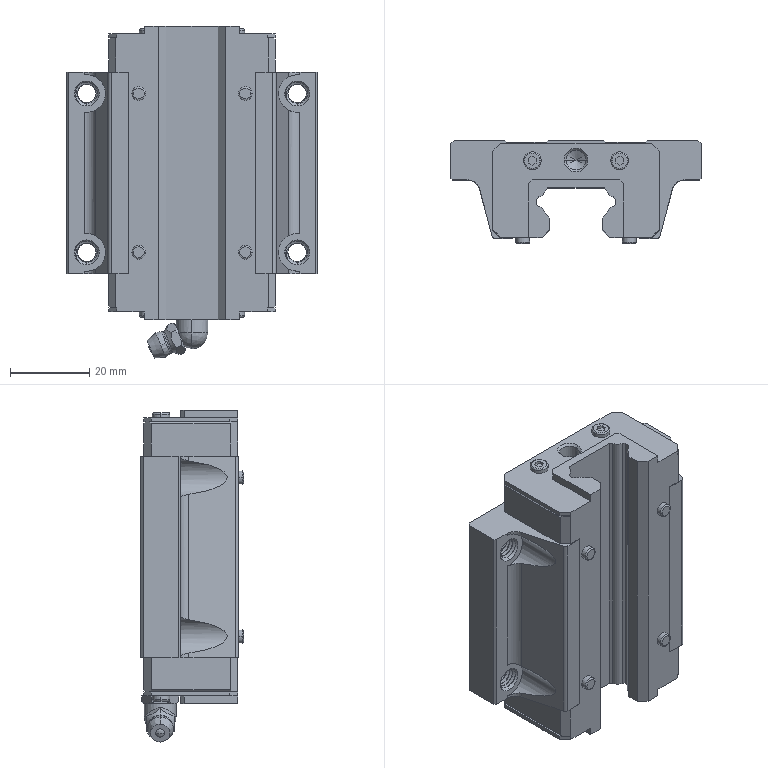Part | SolidWorks | features BaseBody 2 | 2 solids | 365 faces | box 63 x 26 x 83.6 mm | volume 70457 mm3 | plane 162 | cylinder 126 | cone 37 | torus 22 | spline 12 | sphere 6 | commonest cylinder face diameters 6 x92 3.43 x8 4.5 x8 9.5 x6 4.12 x4 4.917 x4